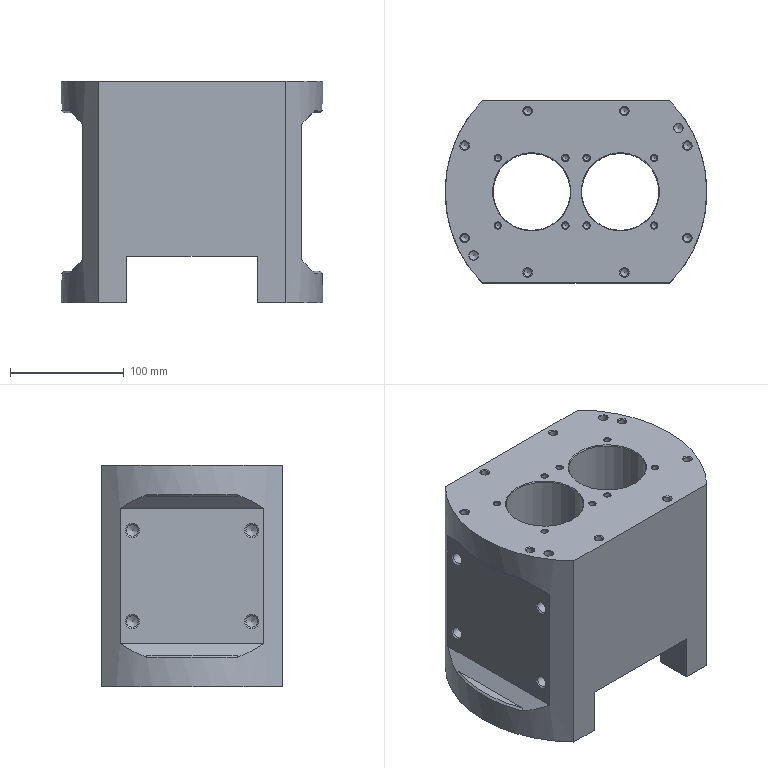NC program | NX | posted with a generic post | part box 230 x 160 x 195 mm
Lines 6467 to 6546 of 6546:
(DRILLING_COPY_1 , TOOL : ZXZ)
N12914 T01 M6
N12916 G54
N12918 G17 G0 G90 X40. Y-52.5 B0. C0. S5000 M3
N12920 G43 Z30. H1
N12922 G94 G81 G98 Z-20. F250. R-16.
N12924 X-40.
N12926 Y52.5
N12928 X40.
N12930 G80
N12932 G0 X40. Y52.5 Z30.
N12934 M5
(DRILLING_COPY_COPY_1 , TOOL : 10.2ZT)
N12936 T11 M6
N12938 G54
N12940 G17 G0 G90 X40. Y-52.5 B0. C0. S1200 M3
N12942 G43 Z30. H11
N12944 G94 G83 G98 Z-48.064 F250. Q2. R-16.
N12946 X-40.
N12948 Y52.5
N12950 X40.
N12952 G80
N12954 G0 X40. Y52.5 Z30.
N12956 M5
(PLANAR_MILL_COPY_COPY_COPY , TOOL : D6A45)
N12958 T07 M6
N12960 G54
N12962 G17 G0 G90 X41.979 Y55.447 B0. C0. S7500 M3
N12964 G43 Z30. H7
N12966 Z-17.5
N12968 G94 G1 Z-20.5 F1250.
N12970 X40.766 Y56.893
N12972 G3 X40. Y57.25 R1.
N12974 X35.25 Y52.5 R4.75
N12976 X40. Y57.25 R-4.75
N12978 X39.234 Y56.893 R1.
N12980 G1 X38.021 Y55.447
N12982 Z-17.5
N12984 G0 Z30.
N12986 X-38.021
N12988 Z-17.5
N12990 G1 Z-20.5
N12992 X-39.234 Y56.893
N12994 G3 X-40. Y57.25 R1.
N12996 X-44.75 Y52.5 R4.75
N12998 X-40. Y57.25 R-4.75
N13000 X-40.766 Y56.893 R1.
N13002 G1 X-41.979 Y55.447
N13004 Z-17.5
N13006 G0 Z30.
N13008 Y-55.447
N13010 Z-17.5
N13012 G1 Z-20.5
N13014 X-40.766 Y-56.893
N13016 G3 X-40. Y-57.25 R1.
N13018 X-35.25 Y-52.5 R4.75
N13020 X-40. Y-57.25 R-4.75
N13022 X-39.234 Y-56.893 R1.
N13024 G1 X-38.021 Y-55.447
N13026 Z-17.5
N13028 G0 Z30.
N13030 X38.021
N13032 Z-17.5
N13034 G1 Z-20.5
N13036 X39.234 Y-56.893
N13038 G3 X40. Y-57.25 R1.
N13040 X44.75 Y-52.5 R4.75
N13042 X40. Y-57.25 R-4.75
N13044 X40.766 Y-56.893 R1.
N13046 G1 X41.979 Y-55.447
N13048 Z-17.5
N13050 G0 Z30.
N13052 M5
N13054 M2